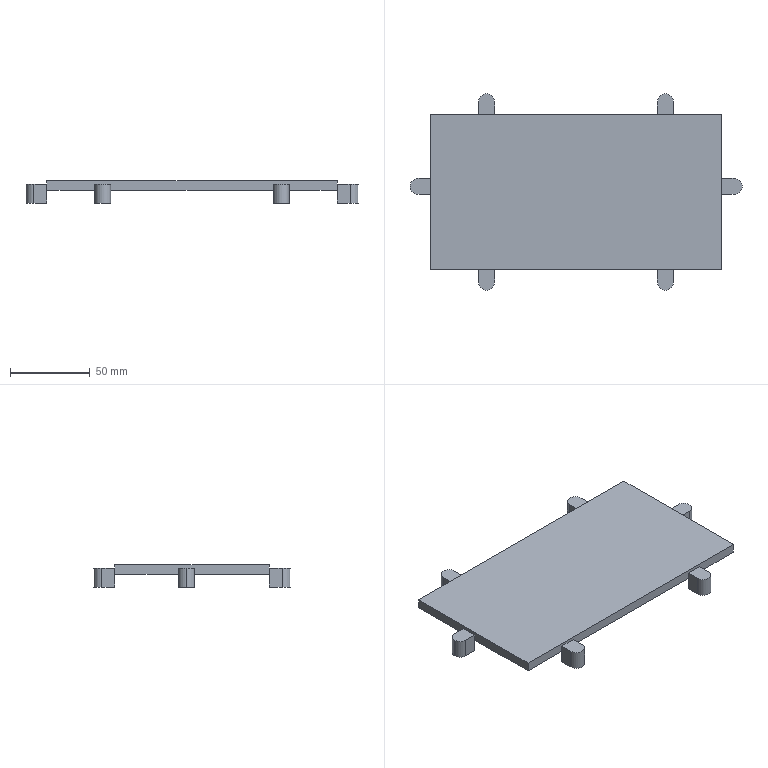Part | SolidWorks | features Extrusion 1, ICE 1 | 1 solid | 43 faces | box 208 x 123 x 14 mm | volume 114511 mm3 | plane 36 | cylinder 7 | commonest cylinder face diameters 10 x7
STEP:
#1=CARTESIAN_POINT('',(-56.993,-5.983,4.));
#2=VERTEX_POINT('',#1);
#3=CARTESIAN_POINT('',(-51.993,-10.983,4.));
#4=VERTEX_POINT('',#3);
#5=CARTESIAN_POINT('',(-51.993,-5.983,4.));
#6=DIRECTION('',(0.,0.,1.));
#7=DIRECTION('',(1.,0.,0.));
#8=AXIS2_PLACEMENT_3D('',#5,#6,#7);
#9=CIRCLE('',#8,5.);
#10=EDGE_CURVE('',#2,#4,#9,.T.);
#11=ORIENTED_EDGE('',*,*,#10,.F.);
#12=CARTESIAN_POINT('',(-56.993,-5.983,-8.));
#13=VERTEX_POINT('',#12);
#14=CARTESIAN_POINT('',(-56.993,-5.983,4.));
#15=DIRECTION('',(0.,0.,-1.));
#16=VECTOR('',#15,1000.);
#17=LINE('',#14,#16);
#18=EDGE_CURVE('',#2,#13,#17,.T.);
#19=ORIENTED_EDGE('',*,*,#18,.T.);
#20=CARTESIAN_POINT('',(-51.993,-10.983,-8.));
#21=VERTEX_POINT('',#20);
#22=CARTESIAN_POINT('',(-51.993,-5.983,-8.));
#23=DIRECTION('',(0.,0.,1.));
#24=DIRECTION('',(1.,0.,0.));
#25=AXIS2_PLACEMENT_3D('',#22,#23,#24);
#26=CIRCLE('',#25,5.);
#27=EDGE_CURVE('',#13,#21,#26,.T.);
#28=ORIENTED_EDGE('',*,*,#27,.T.);
#29=CARTESIAN_POINT('',(-51.993,-10.983,4.));
#30=DIRECTION('',(0.,0.,-1.));
#31=VECTOR('',#30,1000.);
#32=LINE('',#29,#31);
#33=EDGE_CURVE('',#4,#21,#32,.T.);
#34=ORIENTED_EDGE('',*,*,#33,.F.);
#35=EDGE_LOOP('',(#11,#19,#28,#34));
#36=FACE_OUTER_BOUND('',#35,.T.);
#37=CARTESIAN_POINT('',(-51.993,-5.983,4.));
#38=DIRECTION('',(0.,0.,-1.));
#39=DIRECTION('',(-1.,0.,0.));
#40=AXIS2_PLACEMENT_3D('',#37,#38,#39);
#41=CYLINDRICAL_SURFACE('',#40,5.);
#42=ADVANCED_FACE('',(#36),#41,.T.);
#43=CARTESIAN_POINT('',(-13.993,-57.983,4.));
#44=VERTEX_POINT('',#43);
#45=CARTESIAN_POINT('',(-13.993,-57.983,0.));
#46=VERTEX_POINT('',#45);
#47=CARTESIAN_POINT('',(-13.993,-57.983,4.));
#48=DIRECTION('',(0.,0.,-1.));
#49=VECTOR('',#48,1000.);
#50=LINE('',#47,#49);
#51=EDGE_CURVE('',#44,#46,#50,.T.);
#52=ORIENTED_EDGE('',*,*,#51,.F.);
#53=CARTESIAN_POINT('',(-3.993,-57.983,4.));
#54=VERTEX_POINT('',#53);
#55=CARTESIAN_POINT('',(-3.993,-57.983,4.));
#56=DIRECTION('',(-1.,0.,0.));
#57=VECTOR('',#56,1000.);
#58=LINE('',#55,#57);
#59=EDGE_CURVE('',#54,#44,#58,.T.);
#60=ORIENTED_EDGE('',*,*,#59,.F.);
#61=CARTESIAN_POINT('',(-3.993,-57.983,0.));
#62=VERTEX_POINT('',#61);
#63=CARTESIAN_POINT('',(-3.993,-57.983,4.));
#64=DIRECTION('',(0.,0.,-1.));
#65=VECTOR('',#64,1000.);
#66=LINE('',#63,#65);
#67=EDGE_CURVE('',#54,#62,#66,.T.);
#68=ORIENTED_EDGE('',*,*,#67,.T.);
#69=CARTESIAN_POINT('',(98.007,-57.983,0.));
#70=VERTEX_POINT('',#69);
#71=CARTESIAN_POINT('',(138.007,-57.983,0.));
#72=DIRECTION('',(1.,0.,0.));
#73=VECTOR('',#72,1000.);
#74=LINE('',#71,#73);
#75=EDGE_CURVE('',#62,#70,#74,.T.);
#76=ORIENTED_EDGE('',*,*,#75,.T.);
#77=CARTESIAN_POINT('',(98.007,-57.983,4.));
#78=VERTEX_POINT('',#77);
#79=CARTESIAN_POINT('',(98.007,-57.983,4.));
#80=DIRECTION('',(0.,0.,-1.));
#81=VECTOR('',#80,1000.);
#82=LINE('',#79,#81);
#83=EDGE_CURVE('',#78,#70,#82,.T.);
#84=ORIENTED_EDGE('',*,*,#83,.F.);
#85=CARTESIAN_POINT('',(108.007,-57.983,4.));
#86=VERTEX_POINT('',#85);
#87=CARTESIAN_POINT('',(108.007,-57.983,4.));
#88=DIRECTION('',(-1.,0.,0.));
#89=VECTOR('',#88,1000.);
#90=LINE('',#87,#89);
#91=EDGE_CURVE('',#86,#78,#90,.T.);
#92=ORIENTED_EDGE('',*,*,#91,.F.);
#93=CARTESIAN_POINT('',(108.007,-57.983,0.));
#94=VERTEX_POINT('',#93);
#95=CARTESIAN_POINT('',(108.007,-57.983,4.));
#96=DIRECTION('',(0.,0.,-1.));
#97=VECTOR('',#96,1000.);
#98=LINE('',#95,#97);
#99=EDGE_CURVE('',#86,#94,#98,.T.);
#100=ORIENTED_EDGE('',*,*,#99,.T.);
#101=CARTESIAN_POINT('',(138.007,-57.983,0.));
#102=VERTEX_POINT('',#101);
#103=CARTESIAN_POINT('',(138.007,-57.983,0.));
#104=DIRECTION('',(1.,0.,0.));
#105=VECTOR('',#104,1000.);
#106=LINE('',#103,#105);
#107=EDGE_CURVE('',#94,#102,#106,.T.);
#108=ORIENTED_EDGE('',*,*,#107,.T.);
#109=CARTESIAN_POINT('',(138.007,-57.983,6.));
#110=VERTEX_POINT('',#109);
#111=CARTESIAN_POINT('',(138.007,-57.983,6.));
#112=DIRECTION('',(0.,0.,-1.));
#113=VECTOR('',#112,1000.);
#114=LINE('',#111,#113);
#115=EDGE_CURVE('',#110,#102,#114,.T.);
#116=ORIENTED_EDGE('',*,*,#115,.F.);
#117=CARTESIAN_POINT('',(-43.993,-57.983,6.));
#118=VERTEX_POINT('',#117);
#119=CARTESIAN_POINT('',(138.007,-57.983,6.));
#120=DIRECTION('',(1.,0.,0.));
#121=VECTOR('',#120,1000.);
#122=LINE('',#119,#121);
#123=EDGE_CURVE('',#118,#110,#122,.T.);
#124=ORIENTED_EDGE('',*,*,#123,.F.);
#125=CARTESIAN_POINT('',(-43.993,-57.983,0.));
#126=VERTEX_POINT('',#125);
#127=CARTESIAN_POINT('',(-43.993,-57.983,6.));
#128=DIRECTION('',(0.,0.,-1.));
#129=VECTOR('',#128,1000.);
#130=LINE('',#127,#129);
#131=EDGE_CURVE('',#118,#126,#130,.T.);
#132=ORIENTED_EDGE('',*,*,#131,.T.);
#133=CARTESIAN_POINT('',(138.007,-57.983,0.));
#134=DIRECTION('',(1.,0.,0.));
#135=VECTOR('',#134,1000.);
#136=LINE('',#133,#135);
#137=EDGE_CURVE('',#126,#46,#136,.T.);
#138=ORIENTED_EDGE('',*,*,#137,.T.);
#139=EDGE_LOOP('',(#52,#60,#68,#76,#84,#92,#100,#108,#116,#124,#132,#138));
#140=FACE_OUTER_BOUND('',#139,.T.);
#141=CARTESIAN_POINT('',(138.007,-57.983,6.));
#142=DIRECTION('',(0.,1.,0.));
#143=DIRECTION('',(0.,0.,1.));
#144=AXIS2_PLACEMENT_3D('',#141,#142,#143);
#145=PLANE('',#144);
#146=ADVANCED_FACE('',(#140),#145,.F.);
#147=CARTESIAN_POINT('',(-43.993,-0.9829,4.));
#148=VERTEX_POINT('',#147);
#149=CARTESIAN_POINT('',(-43.993,-0.9829,0.));
#150=VERTEX_POINT('',#149);
#151=CARTESIAN_POINT('',(-43.993,-0.9829,4.));
#152=DIRECTION('',(0.,0.,-1.));
#153=VECTOR('',#152,1000.);
#154=LINE('',#151,#153);
#155=EDGE_CURVE('',#148,#150,#154,.T.);
#156=ORIENTED_EDGE('',*,*,#155,.F.);
#157=CARTESIAN_POINT('',(-43.993,-10.983,4.));
#158=VERTEX_POINT('',#157);
#159=CARTESIAN_POINT('',(-43.993,-10.983,4.));
#160=DIRECTION('',(0.,1.,0.));
#161=VECTOR('',#160,1000.);
#162=LINE('',#159,#161);
#163=EDGE_CURVE('',#158,#148,#162,.T.);
#164=ORIENTED_EDGE('',*,*,#163,.F.);
#165=CARTESIAN_POINT('',(-43.993,-10.983,0.));
#166=VERTEX_POINT('',#165);
#167=CARTESIAN_POINT('',(-43.993,-10.983,4.));
#168=DIRECTION('',(0.,0.,-1.));
#169=VECTOR('',#168,1000.);
#170=LINE('',#167,#169);
#171=EDGE_CURVE('',#158,#166,#170,.T.);
#172=ORIENTED_EDGE('',*,*,#171,.T.);
#173=CARTESIAN_POINT('',(-43.993,-57.983,0.));
#174=DIRECTION('',(0.,-1.,0.));
#175=VECTOR('',#174,1000.);
#176=LINE('',#173,#175);
#177=EDGE_CURVE('',#166,#126,#176,.T.);
#178=ORIENTED_EDGE('',*,*,#177,.T.);
#179=ORIENTED_EDGE('',*,*,#131,.F.);
#180=CARTESIAN_POINT('',(-43.993,39.017,6.));
#181=VERTEX_POINT('',#180);
#182=CARTESIAN_POINT('',(-43.993,-57.983,6.));
#183=DIRECTION('',(0.,-1.,0.));
#184=VECTOR('',#183,1000.);
#185=LINE('',#182,#184);
#186=EDGE_CURVE('',#181,#118,#185,.T.);
#187=ORIENTED_EDGE('',*,*,#186,.F.);
#188=CARTESIAN_POINT('',(-43.993,39.017,0.));
#189=VERTEX_POINT('',#188);
#190=CARTESIAN_POINT('',(-43.993,39.017,6.));
#191=DIRECTION('',(0.,0.,-1.));
#192=VECTOR('',#191,1000.);
#193=LINE('',#190,#192);
#194=EDGE_CURVE('',#181,#189,#193,.T.);
#195=ORIENTED_EDGE('',*,*,#194,.T.);
#196=CARTESIAN_POINT('',(-43.993,-57.983,0.));
#197=DIRECTION('',(0.,-1.,0.));
#198=VECTOR('',#197,1000.);
#199=LINE('',#196,#198);
#200=EDGE_CURVE('',#189,#150,#199,.T.);
#201=ORIENTED_EDGE('',*,*,#200,.T.);
#202=EDGE_LOOP('',(#156,#164,#172,#178,#179,#187,#195,#201));
#203=FACE_OUTER_BOUND('',#202,.T.);
#204=CARTESIAN_POINT('',(-43.993,-57.983,6.));
#205=DIRECTION('',(1.,0.,0.));
#206=DIRECTION('',(0.,0.,-1.));
#207=AXIS2_PLACEMENT_3D('',#204,#205,#206);
#208=PLANE('',#207);
#209=ADVANCED_FACE('',(#203),#208,.F.);
#210=CARTESIAN_POINT('',(108.007,39.017,4.));
#211=VERTEX_POINT('',#210);
#212=CARTESIAN_POINT('',(108.007,39.017,0.));
#213=VERTEX_POINT('',#212);
#214=CARTESIAN_POINT('',(108.007,39.017,4.));
#215=DIRECTION('',(0.,0.,-1.));
#216=VECTOR('',#215,1000.);
#217=LINE('',#214,#216);
#218=EDGE_CURVE('',#211,#213,#217,.T.);
#219=ORIENTED_EDGE('',*,*,#218,.F.);
#220=CARTESIAN_POINT('',(98.007,39.017,4.));
#221=VERTEX_POINT('',#220);
#222=CARTESIAN_POINT('',(98.007,39.017,4.));
#223=DIRECTION('',(1.,0.,0.));
#224=VECTOR('',#223,1000.);
#225=LINE('',#222,#224);
#226=EDGE_CURVE('',#221,#211,#225,.T.);
#227=ORIENTED_EDGE('',*,*,#226,.F.);
#228=CARTESIAN_POINT('',(98.007,39.017,0.));
#229=VERTEX_POINT('',#228);
#230=CARTESIAN_POINT('',(98.007,39.017,4.));
#231=DIRECTION('',(0.,0.,-1.));
#232=VECTOR('',#231,1000.);
#233=LINE('',#230,#232);
#234=EDGE_CURVE('',#221,#229,#233,.T.);
#235=ORIENTED_EDGE('',*,*,#234,.T.);
#236=CARTESIAN_POINT('',(-3.993,39.017,0.));
#237=VERTEX_POINT('',#236);
#238=CARTESIAN_POINT('',(138.007,39.017,0.));
#239=DIRECTION('',(-1.,0.,0.));
#240=VECTOR('',#239,1000.);
#241=LINE('',#238,#240);
#242=EDGE_CURVE('',#229,#237,#241,.T.);
#243=ORIENTED_EDGE('',*,*,#242,.T.);
#244=CARTESIAN_POINT('',(-3.993,39.017,4.));
#245=VERTEX_POINT('',#244);
#246=CARTESIAN_POINT('',(-3.993,39.017,4.));
#247=DIRECTION('',(0.,0.,-1.));
#248=VECTOR('',#247,1000.);
#249=LINE('',#246,#248);
#250=EDGE_CURVE('',#245,#237,#249,.T.);
#251=ORIENTED_EDGE('',*,*,#250,.F.);
#252=CARTESIAN_POINT('',(-13.993,39.017,4.));
#253=VERTEX_POINT('',#252);
#254=CARTESIAN_POINT('',(-13.993,39.017,4.));
#255=DIRECTION('',(1.,0.,0.));
#256=VECTOR('',#255,1000.);
#257=LINE('',#254,#256);
#258=EDGE_CURVE('',#253,#245,#257,.T.);
#259=ORIENTED_EDGE('',*,*,#258,.F.);
#260=CARTESIAN_POINT('',(-13.993,39.017,0.));
#261=VERTEX_POINT('',#260);
#262=CARTESIAN_POINT('',(-13.993,39.017,4.));
#263=DIRECTION('',(0.,0.,-1.));
#264=VECTOR('',#263,1000.);
#265=LINE('',#262,#264);
#266=EDGE_CURVE('',#253,#261,#265,.T.);
#267=ORIENTED_EDGE('',*,*,#266,.T.);
#268=CARTESIAN_POINT('',(138.007,39.017,0.));
#269=DIRECTION('',(-1.,0.,0.));
#270=VECTOR('',#269,1000.);
#271=LINE('',#268,#270);
#272=EDGE_CURVE('',#261,#189,#271,.T.);
#273=ORIENTED_EDGE('',*,*,#272,.T.);
#274=ORIENTED_EDGE('',*,*,#194,.F.);
#275=CARTESIAN_POINT('',(138.007,39.017,6.));
#276=VERTEX_POINT('',#275);
#277=CARTESIAN_POINT('',(138.007,39.017,6.));
#278=DIRECTION('',(-1.,0.,0.));
#279=VECTOR('',#278,1000.);
#280=LINE('',#277,#279);
#281=EDGE_CURVE('',#276,#181,#280,.T.);
#282=ORIENTED_EDGE('',*,*,#281,.F.);
#283=CARTESIAN_POINT('',(138.007,39.017,0.));
#284=VERTEX_POINT('',#283);
#285=CARTESIAN_POINT('',(138.007,39.017,6.));
#286=DIRECTION('',(0.,0.,-1.));
#287=VECTOR('',#286,1000.);
#288=LINE('',#285,#287);
#289=EDGE_CURVE('',#276,#284,#288,.T.);
#290=ORIENTED_EDGE('',*,*,#289,.T.);
#291=CARTESIAN_POINT('',(138.007,39.017,0.));
#292=DIRECTION('',(-1.,0.,0.));
#293=VECTOR('',#292,1000.);
#294=LINE('',#291,#293);
#295=EDGE_CURVE('',#284,#213,#294,.T.);
#296=ORIENTED_EDGE('',*,*,#295,.T.);
#297=EDGE_LOOP('',(#219,#227,#235,#243,#251,#259,#267,#273,#274,#282,#290,#296));
#298=FACE_OUTER_BOUND('',#297,.T.);
#299=CARTESIAN_POINT('',(138.007,39.017,6.));
#300=DIRECTION('',(0.,-1.,0.));
#301=DIRECTION('',(0.,0.,-1.));
#302=AXIS2_PLACEMENT_3D('',#299,#300,#301);
#303=PLANE('',#302);
#304=ADVANCED_FACE('',(#298),#303,.F.);
#305=CARTESIAN_POINT('',(138.007,-10.983,4.));
#306=VERTEX_POINT('',#305);
#307=CARTESIAN_POINT('',(138.007,-10.983,0.));
#308=VERTEX_POINT('',#307);
#309=CARTESIAN_POINT('',(138.007,-10.983,4.));
#310=DIRECTION('',(0.,0.,-1.));
#311=VECTOR('',#310,1000.);
#312=LINE('',#309,#311);
#313=EDGE_CURVE('',#306,#308,#312,.T.);
#314=ORIENTED_EDGE('',*,*,#313,.F.);
#315=CARTESIAN_POINT('',(138.007,-0.9829,4.));
#316=VERTEX_POINT('',#315);
#317=CARTESIAN_POINT('',(138.007,-0.9829,4.));
#318=DIRECTION('',(0.,-1.,0.));
#319=VECTOR('',#318,1000.);
#320=LINE('',#317,#319);
#321=EDGE_CURVE('',#316,#306,#320,.T.);
#322=ORIENTED_EDGE('',*,*,#321,.F.);
#323=CARTESIAN_POINT('',(138.007,-0.9829,0.));
#324=VERTEX_POINT('',#323);
#325=CARTESIAN_POINT('',(138.007,-0.9829,4.));
#326=DIRECTION('',(0.,0.,-1.));
#327=VECTOR('',#326,1000.);
#328=LINE('',#325,#327);
#329=EDGE_CURVE('',#316,#324,#328,.T.);
#330=ORIENTED_EDGE('',*,*,#329,.T.);
#331=CARTESIAN_POINT('',(138.007,-57.983,0.));
#332=DIRECTION('',(0.,1.,0.));
#333=VECTOR('',#332,1000.);
#334=LINE('',#331,#333);
#335=EDGE_CURVE('',#324,#284,#334,.T.);
#336=ORIENTED_EDGE('',*,*,#335,.T.);
#337=ORIENTED_EDGE('',*,*,#289,.F.);
#338=CARTESIAN_POINT('',(138.007,-57.983,6.));
#339=DIRECTION('',(0.,1.,0.));
#340=VECTOR('',#339,1000.);
#341=LINE('',#338,#340);
#342=EDGE_CURVE('',#110,#276,#341,.T.);
#343=ORIENTED_EDGE('',*,*,#342,.F.);
#344=ORIENTED_EDGE('',*,*,#115,.T.);
#345=CARTESIAN_POINT('',(138.007,-57.983,0.));
#346=DIRECTION('',(0.,1.,0.));
#347=VECTOR('',#346,1000.);
#348=LINE('',#345,#347);
#349=EDGE_CURVE('',#102,#308,#348,.T.);
#350=ORIENTED_EDGE('',*,*,#349,.T.);
#351=EDGE_LOOP('',(#314,#322,#330,#336,#337,#343,#344,#350));
#352=FACE_OUTER_BOUND('',#351,.T.);
#353=CARTESIAN_POINT('',(138.007,-57.983,6.));
#354=DIRECTION('',(-1.,0.,0.));
#355=DIRECTION('',(0.,0.,1.));
#356=AXIS2_PLACEMENT_3D('',#353,#354,#355);
#357=PLANE('',#356);
#358=ADVANCED_FACE('',(#352),#357,.F.);
#359=ORIENTED_EDGE('',*,*,#342,.T.);
#360=ORIENTED_EDGE('',*,*,#281,.T.);
#361=ORIENTED_EDGE('',*,*,#186,.T.);
#362=ORIENTED_EDGE('',*,*,#123,.T.);
#363=EDGE_LOOP('',(#359,#360,#361,#362));
#364=FACE_OUTER_BOUND('',#363,.T.);
#365=CARTESIAN_POINT('',(0.,0.,6.));
#366=DIRECTION('',(0.,0.,1.));
#367=DIRECTION('',(1.,0.,0.));
#368=AXIS2_PLACEMENT_3D('',#365,#366,#367);
#369=PLANE('',#368);
#370=ADVANCED_FACE('',(#364),#369,.T.);
#371=ORIENTED_EDGE('',*,*,#349,.F.);
#372=ORIENTED_EDGE('',*,*,#107,.F.);
#373=CARTESIAN_POINT('',(138.007,-57.983,0.));
#374=DIRECTION('',(1.,0.,0.));
#375=VECTOR('',#374,1000.);
#376=LINE('',#373,#375);
#377=EDGE_CURVE('',#70,#94,#376,.T.);
#378=ORIENTED_EDGE('',*,*,#377,.F.);
#379=ORIENTED_EDGE('',*,*,#75,.F.);
#380=CARTESIAN_POINT('',(138.007,-57.983,0.));
#381=DIRECTION('',(1.,0.,0.));
#382=VECTOR('',#381,1000.);
#383=LINE('',#380,#382);
#384=EDGE_CURVE('',#46,#62,#383,.T.);
#385=ORIENTED_EDGE('',*,*,#384,.F.);
#386=ORIENTED_EDGE('',*,*,#137,.F.);
#387=ORIENTED_EDGE('',*,*,#177,.F.);
#388=CARTESIAN_POINT('',(-43.993,-57.983,0.));
#389=DIRECTION('',(0.,-1.,0.));
#390=VECTOR('',#389,1000.);
#391=LINE('',#388,#390);
#392=EDGE_CURVE('',#150,#166,#391,.T.);
#393=ORIENTED_EDGE('',*,*,#392,.F.);
#394=ORIENTED_EDGE('',*,*,#200,.F.);
#395=ORIENTED_EDGE('',*,*,#272,.F.);
#396=CARTESIAN_POINT('',(138.007,39.017,0.));
#397=DIRECTION('',(-1.,0.,0.));
#398=VECTOR('',#397,1000.);
#399=LINE('',#396,#398);
#400=EDGE_CURVE('',#237,#261,#399,.T.);
#401=ORIENTED_EDGE('',*,*,#400,.F.);
#402=ORIENTED_EDGE('',*,*,#242,.F.);
#403=CARTESIAN_POINT('',(138.007,39.017,0.));
#404=DIRECTION('',(-1.,0.,0.));
#405=VECTOR('',#404,1000.);
#406=LINE('',#403,#405);
#407=EDGE_CURVE('',#213,#229,#406,.T.);
#408=ORIENTED_EDGE('',*,*,#407,.F.);
#409=ORIENTED_EDGE('',*,*,#295,.F.);
#410=ORIENTED_EDGE('',*,*,#335,.F.);
#411=CARTESIAN_POINT('',(138.007,-57.983,0.));
#412=DIRECTION('',(0.,1.,0.));
#413=VECTOR('',#412,1000.);
#414=LINE('',#411,#413);
#415=EDGE_CURVE('',#308,#324,#414,.T.);
#416=ORIENTED_EDGE('',*,*,#415,.F.);
#417=EDGE_LOOP('',(#371,#372,#378,#379,#385,#386,#387,#393,#394,#395,#401,#402,#408,#409,#410,#416));
#418=FACE_OUTER_BOUND('',#417,.T.);
#419=CARTESIAN_POINT('',(0.,0.,0.));
#420=DIRECTION('',(0.,0.,1.));
#421=DIRECTION('',(1.,0.,0.));
#422=AXIS2_PLACEMENT_3D('',#419,#420,#421);
#423=PLANE('',#422);
#424=ADVANCED_FACE('',(#418),#423,.F.);
#425=CARTESIAN_POINT('',(98.007,-57.983,-8.));
#426=VERTEX_POINT('',#425);
#427=CARTESIAN_POINT('',(98.007,-57.983,4.));
#428=DIRECTION('',(0.,0.,-1.));
#429=VECTOR('',#428,1000.);
#430=LINE('',#427,#429);
#431=EDGE_CURVE('',#70,#426,#430,.T.);
#432=ORIENTED_EDGE('',*,*,#431,.F.);
#433=ORIENTED_EDGE('',*,*,#377,.T.);
#434=CARTESIAN_POINT('',(108.007,-57.983,-8.));
#435=VERTEX_POINT('',#434);
#436=CARTESIAN_POINT('',(108.007,-57.983,4.));
#437=DIRECTION('',(0.,0.,-1.));
#438=VECTOR('',#437,1000.);
#439=LINE('',#436,#438);
#440=EDGE_CURVE('',#94,#435,#439,.T.);
#441=ORIENTED_EDGE('',*,*,#440,.T.);
#442=CARTESIAN_POINT('',(108.007,-57.983,-8.));
#443=DIRECTION('',(-1.,0.,0.));
#444=VECTOR('',#443,1000.);
#445=LINE('',#442,#444);
#446=EDGE_CURVE('',#435,#426,#445,.T.);
#447=ORIENTED_EDGE('',*,*,#446,.T.);
#448=EDGE_LOOP('',(#432,#433,#441,#447));
#449=FACE_OUTER_BOUND('',#448,.T.);
#450=CARTESIAN_POINT('',(108.007,-57.983,4.));
#451=DIRECTION('',(0.,-1.,0.));
#452=DIRECTION('',(0.,0.,-1.));
#453=AXIS2_PLACEMENT_3D('',#450,#451,#452);
#454=PLANE('',#453);
#455=ADVANCED_FACE('',(#449),#454,.F.);
#456=CARTESIAN_POINT('',(98.007,-65.983,-8.));
#457=VERTEX_POINT('',#456);
#458=CARTESIAN_POINT('',(108.007,-65.983,-8.));
#459=VERTEX_POINT('',#458);
#460=CARTESIAN_POINT('',(103.007,-65.983,-8.));
#461=DIRECTION('',(0.,0.,1.));
#462=DIRECTION('',(1.,0.,0.));
#463=AXIS2_PLACEMENT_3D('',#460,#461,#462);
#464=CIRCLE('',#463,5.);
#465=EDGE_CURVE('',#457,#459,#464,.T.);
#466=ORIENTED_EDGE('',*,*,#465,.T.);
#467=CARTESIAN_POINT('',(108.007,-65.983,4.));
#468=VERTEX_POINT('',#467);
#469=CARTESIAN_POINT('',(108.007,-65.983,4.));
#470=DIRECTION('',(0.,0.,-1.));
#471=VECTOR('',#470,1000.);
#472=LINE('',#469,#471);
#473=EDGE_CURVE('',#468,#459,#472,.T.);
#474=ORIENTED_EDGE('',*,*,#473,.F.);
#475=CARTESIAN_POINT('',(98.007,-65.983,4.));
#476=VERTEX_POINT('',#475);
#477=CARTESIAN_POINT('',(103.007,-65.983,4.));
#478=DIRECTION('',(0.,0.,1.));
#479=DIRECTION('',(1.,0.,0.));
#480=AXIS2_PLACEMENT_3D('',#477,#478,#479);
#481=CIRCLE('',#480,5.);
#482=EDGE_CURVE('',#476,#468,#481,.T.);
#483=ORIENTED_EDGE('',*,*,#482,.F.);
#484=CARTESIAN_POINT('',(98.007,-65.983,4.));
#485=DIRECTION('',(0.,0.,-1.));
#486=VECTOR('',#485,1000.);
#487=LINE('',#484,#486);
#488=EDGE_CURVE('',#476,#457,#487,.T.);
#489=ORIENTED_EDGE('',*,*,#488,.T.);
#490=EDGE_LOOP('',(#466,#474,#483,#489));
#491=FACE_OUTER_BOUND('',#490,.T.);
#492=CARTESIAN_POINT('',(103.007,-65.983,4.));
#493=DIRECTION('',(0.,0.,-1.));
#494=DIRECTION('',(-1.,0.,0.));
#495=AXIS2_PLACEMENT_3D('',#492,#493,#494);
#496=CYLINDRICAL_SURFACE('',#495,5.);
#497=ADVANCED_FACE('',(#491),#496,.T.);
#498=CARTESIAN_POINT('',(108.007,-65.983,-8.));
#499=DIRECTION('',(0.,1.,0.));
#500=VECTOR('',#499,1000.);
#501=LINE('',#498,#500);
#502=EDGE_CURVE('',#459,#435,#501,.T.);
#503=ORIENTED_EDGE('',*,*,#502,.T.);
#504=ORIENTED_EDGE('',*,*,#440,.F.);
#505=ORIENTED_EDGE('',*,*,#99,.F.);
#506=CARTESIAN_POINT('',(108.007,-65.983,4.));
#507=DIRECTION('',(0.,1.,0.));
#508=VECTOR('',#507,1000.);
#509=LINE('',#506,#508);
#510=EDGE_CURVE('',#468,#86,#509,.T.);
#511=ORIENTED_EDGE('',*,*,#510,.F.);
#512=ORIENTED_EDGE('',*,*,#473,.T.);
#513=EDGE_LOOP('',(#503,#504,#505,#511,#512));
#514=FACE_OUTER_BOUND('',#513,.T.);
#515=CARTESIAN_POINT('',(108.007,-65.983,4.));
#516=DIRECTION('',(-1.,0.,0.));
#517=DIRECTION('',(0.,-1.,0.));
#518=AXIS2_PLACEMENT_3D('',#515,#516,#517);
#519=PLANE('',#518);
#520=ADVANCED_FACE('',(#514),#519,.F.);
#521=CARTESIAN_POINT('',(98.007,-57.983,-8.));
#522=DIRECTION('',(0.,-1.,0.));
#523=VECTOR('',#522,1000.);
#524=LINE('',#521,#523);
#525=EDGE_CURVE('',#426,#457,#524,.T.);
#526=ORIENTED_EDGE('',*,*,#525,.T.);
#527=ORIENTED_EDGE('',*,*,#488,.F.);
#528=CARTESIAN_POINT('',(98.007,-57.983,4.));
#529=DIRECTION('',(0.,-1.,0.));
#530=VECTOR('',#529,1000.);
#531=LINE('',#528,#530);
#532=EDGE_CURVE('',#78,#476,#531,.T.);
#533=ORIENTED_EDGE('',*,*,#532,.F.);
#534=ORIENTED_EDGE('',*,*,#83,.T.);
#535=ORIENTED_EDGE('',*,*,#431,.T.);
#536=EDGE_LOOP('',(#526,#527,#533,#534,#535));
#537=FACE_OUTER_BOUND('',#536,.T.);
#538=CARTESIAN_POINT('',(98.007,-57.983,4.));
#539=DIRECTION('',(1.,0.,0.));
#540=DIRECTION('',(0.,1.,0.));
#541=AXIS2_PLACEMENT_3D('',#538,#539,#540);
#542=PLANE('',#541);
#543=ADVANCED_FACE('',(#537),#542,.F.);
#544=ORIENTED_EDGE('',*,*,#482,.T.);
#545=ORIENTED_EDGE('',*,*,#510,.T.);
#546=ORIENTED_EDGE('',*,*,#91,.T.);
#547=ORIENTED_EDGE('',*,*,#532,.T.);
#548=EDGE_LOOP('',(#544,#545,#546,#547));
#549=FACE_OUTER_BOUND('',#548,.T.);
#550=CARTESIAN_POINT('',(103.007,-65.983,4.));
#551=DIRECTION('',(0.,0.,1.));
#552=DIRECTION('',(1.,0.,0.));
#553=AXIS2_PLACEMENT_3D('',#550,#551,#552);
#554=PLANE('',#553);
#555=ADVANCED_FACE('',(#549),#554,.T.);
#556=ORIENTED_EDGE('',*,*,#465,.F.);
#557=ORIENTED_EDGE('',*,*,#525,.F.);
#558=ORIENTED_EDGE('',*,*,#446,.F.);
#559=ORIENTED_EDGE('',*,*,#502,.F.);
#560=EDGE_LOOP('',(#556,#557,#558,#559));
#561=FACE_OUTER_BOUND('',#560,.T.);
#562=CARTESIAN_POINT('',(103.007,-65.983,-8.));
#563=DIRECTION('',(0.,0.,1.));
#564=DIRECTION('',(1.,0.,0.));
#565=AXIS2_PLACEMENT_3D('',#562,#563,#564);
#566=PLANE('',#565);
#567=ADVANCED_FACE('',(#561),#566,.F.);
#568=CARTESIAN_POINT('',(138.007,-10.983,-8.));
#569=VERTEX_POINT('',#568);
#570=CARTESIAN_POINT('',(138.007,-10.983,4.));
#571=DIRECTION('',(0.,0.,-1.));
#572=VECTOR('',#571,1000.);
#573=LINE('',#570,#572);
#574=EDGE_CURVE('',#308,#569,#573,.T.);
#575=ORIENTED_EDGE('',*,*,#574,.F.);
#576=ORIENTED_EDGE('',*,*,#415,.T.);
#577=CARTESIAN_POINT('',(138.007,-0.9829,-8.));
#578=VERTEX_POINT('',#577);
#579=CARTESIAN_POINT('',(138.007,-0.9829,4.));
#580=DIRECTION('',(0.,0.,-1.));
#581=VECTOR('',#580,1000.);
#582=LINE('',#579,#581);
#583=EDGE_CURVE('',#324,#578,#582,.T.);
#584=ORIENTED_EDGE('',*,*,#583,.T.);
#585=CARTESIAN_POINT('',(138.007,-0.9829,-8.));
#586=DIRECTION('',(0.,-1.,0.));
#587=VECTOR('',#586,1000.);
#588=LINE('',#585,#587);
#589=EDGE_CURVE('',#578,#569,#588,.T.);
#590=ORIENTED_EDGE('',*,*,#589,.T.);
#591=EDGE_LOOP('',(#575,#576,#584,#590));
#592=FACE_OUTER_BOUND('',#591,.T.);
#593=CARTESIAN_POINT('',(138.007,-0.9829,4.));
#594=DIRECTION('',(1.,0.,0.));
#595=DIRECTION('',(0.,0.,-1.));
#596=AXIS2_PLACEMENT_3D('',#593,#594,#595);
#597=PLANE('',#596);
#598=ADVANCED_FACE('',(#592),#597,.F.);
#599=CARTESIAN_POINT('',(146.007,-0.9829,-8.));
#600=VERTEX_POINT('',#599);
#601=CARTESIAN_POINT('',(146.007,-0.9829,-8.));
#602=DIRECTION('',(-1.,0.,0.));
#603=VECTOR('',#602,1000.);
#604=LINE('',#601,#603);
#605=EDGE_CURVE('',#600,#578,#604,.T.);
#606=ORIENTED_EDGE('',*,*,#605,.T.);
#607=ORIENTED_EDGE('',*,*,#583,.F.);
#608=ORIENTED_EDGE('',*,*,#329,.F.);
#609=CARTESIAN_POINT('',(146.007,-0.9829,4.));
#610=VERTEX_POINT('',#609);
#611=CARTESIAN_POINT('',(146.007,-0.9829,4.));
#612=DIRECTION('',(-1.,0.,0.));
#613=VECTOR('',#612,1000.);
#614=LINE('',#611,#613);
#615=EDGE_CURVE('',#610,#316,#614,.T.);
#616=ORIENTED_EDGE('',*,*,#615,.F.);
#617=CARTESIAN_POINT('',(146.007,-0.9829,4.));
#618=DIRECTION('',(0.,0.,-1.));
#619=VECTOR('',#618,1000.);
#620=LINE('',#617,#619);
#621=EDGE_CURVE('',#610,#600,#620,.T.);
#622=ORIENTED_EDGE('',*,*,#621,.T.);
#623=EDGE_LOOP('',(#606,#607,#608,#616,#622));
#624=FACE_OUTER_BOUND('',#623,.T.);
#625=CARTESIAN_POINT('',(146.007,-0.9829,4.));
#626=DIRECTION('',(0.,-1.,0.));
#627=DIRECTION('',(0.,0.,-1.));
#628=AXIS2_PLACEMENT_3D('',#625,#626,#627);
#629=PLANE('',#628);
#630=ADVANCED_FACE('',(#624),#629,.F.);
#631=CARTESIAN_POINT('',(146.007,-10.983,-8.));
#632=VERTEX_POINT('',#631);
#633=CARTESIAN_POINT('',(138.007,-10.983,-8.));
#634=DIRECTION('',(1.,0.,0.));
#635=VECTOR('',#634,1000.);
#636=LINE('',#633,#635);
#637=EDGE_CURVE('',#569,#632,#636,.T.);
#638=ORIENTED_EDGE('',*,*,#637,.T.);
#639=CARTESIAN_POINT('',(146.007,-10.983,4.));
#640=VERTEX_POINT('',#639);
#641=CARTESIAN_POINT('',(146.007,-10.983,4.));
#642=DIRECTION('',(0.,0.,-1.));
#643=VECTOR('',#642,1000.);
#644=LINE('',#641,#643);
#645=EDGE_CURVE('',#640,#632,#644,.T.);
#646=ORIENTED_EDGE('',*,*,#645,.F.);
#647=CARTESIAN_POINT('',(138.007,-10.983,4.));
#648=DIRECTION('',(1.,0.,0.));
#649=VECTOR('',#648,1000.);
#650=LINE('',#647,#649);
#651=EDGE_CURVE('',#306,#640,#650,.T.);
#652=ORIENTED_EDGE('',*,*,#651,.F.);
#653=ORIENTED_EDGE('',*,*,#313,.T.);
#654=ORIENTED_EDGE('',*,*,#574,.T.);
#655=EDGE_LOOP('',(#638,#646,#652,#653,#654));
#656=FACE_OUTER_BOUND('',#655,.T.);
#657=CARTESIAN_POINT('',(138.007,-10.983,4.));
#658=DIRECTION('',(0.,1.,0.));
#659=DIRECTION('',(-1.,0.,0.));
#660=AXIS2_PLACEMENT_3D('',#657,#658,#659);
#661=PLANE('',#660);
#662=ADVANCED_FACE('',(#656),#661,.F.);
#663=CARTESIAN_POINT('',(146.007,-5.983,-8.));
#664=DIRECTION('',(0.,0.,1.));
#665=DIRECTION('',(1.,0.,0.));
#666=AXIS2_PLACEMENT_3D('',#663,#664,#665);
#667=CIRCLE('',#666,5.);
#668=EDGE_CURVE('',#632,#600,#667,.T.);
#669=ORIENTED_EDGE('',*,*,#668,.T.);
#670=ORIENTED_EDGE('',*,*,#621,.F.);
#671=CARTESIAN_POINT('',(146.007,-5.983,4.));
#672=DIRECTION('',(0.,0.,1.));
#673=DIRECTION('',(1.,0.,0.));
#674=AXIS2_PLACEMENT_3D('',#671,#672,#673);
#675=CIRCLE('',#674,5.);
#676=EDGE_CURVE('',#640,#610,#675,.T.);
#677=ORIENTED_EDGE('',*,*,#676,.F.);
#678=ORIENTED_EDGE('',*,*,#645,.T.);
#679=EDGE_LOOP('',(#669,#670,#677,#678));
#680=FACE_OUTER_BOUND('',#679,.T.);
#681=CARTESIAN_POINT('',(146.007,-5.983,4.));
#682=DIRECTION('',(0.,0.,-1.));
#683=DIRECTION('',(-1.,0.,0.));
#684=AXIS2_PLACEMENT_3D('',#681,#682,#683);
#685=CYLINDRICAL_SURFACE('',#684,5.);
#686=ADVANCED_FACE('',(#680),#685,.T.);
#687=ORIENTED_EDGE('',*,*,#615,.T.);
#688=ORIENTED_EDGE('',*,*,#321,.T.);
#689=ORIENTED_EDGE('',*,*,#651,.T.);
#690=ORIENTED_EDGE('',*,*,#676,.T.);
#691=EDGE_LOOP('',(#687,#688,#689,#690));
#692=FACE_OUTER_BOUND('',#691,.T.);
#693=CARTESIAN_POINT('',(146.007,-5.983,4.));
#694=DIRECTION('',(0.,0.,1.));
#695=DIRECTION('',(1.,0.,0.));
#696=AXIS2_PLACEMENT_3D('',#693,#694,#695);
#697=PLANE('',#696);
#698=ADVANCED_FACE('',(#692),#697,.T.);
#699=ORIENTED_EDGE('',*,*,#605,.F.);
#700=ORIENTED_EDGE('',*,*,#668,.F.);
#701=ORIENTED_EDGE('',*,*,#637,.F.);
#702=ORIENTED_EDGE('',*,*,#589,.F.);
#703=EDGE_LOOP('',(#699,#700,#701,#702));
#704=FACE_OUTER_BOUND('',#703,.T.);
#705=CARTESIAN_POINT('',(146.007,-5.983,-8.));
#706=DIRECTION('',(0.,0.,1.));
#707=DIRECTION('',(1.,0.,0.));
#708=AXIS2_PLACEMENT_3D('',#705,#706,#707);
#709=PLANE('',#708);
#710=ADVANCED_FACE('',(#704),#709,.F.);
#711=CARTESIAN_POINT('',(-3.993,39.017,-8.));
#712=VERTEX_POINT('',#711);
#713=CARTESIAN_POINT('',(-3.993,39.017,4.));
#714=DIRECTION('',(0.,0.,-1.));
#715=VECTOR('',#714,1000.);
#716=LINE('',#713,#715);
#717=EDGE_CURVE('',#237,#712,#716,.T.);
#718=ORIENTED_EDGE('',*,*,#717,.F.);
#719=ORIENTED_EDGE('',*,*,#400,.T.);
#720=CARTESIAN_POINT('',(-13.993,39.017,-8.));
#721=VERTEX_POINT('',#720);
#722=CARTESIAN_POINT('',(-13.993,39.017,4.));
#723=DIRECTION('',(0.,0.,-1.));
#724=VECTOR('',#723,1000.);
#725=LINE('',#722,#724);
#726=EDGE_CURVE('',#261,#721,#725,.T.);
#727=ORIENTED_EDGE('',*,*,#726,.T.);
#728=CARTESIAN_POINT('',(-13.993,39.017,-8.));
#729=DIRECTION('',(1.,0.,0.));
#730=VECTOR('',#729,1000.);
#731=LINE('',#728,#730);
#732=EDGE_CURVE('',#721,#712,#731,.T.);
#733=ORIENTED_EDGE('',*,*,#732,.T.);
#734=EDGE_LOOP('',(#718,#719,#727,#733));
#735=FACE_OUTER_BOUND('',#734,.T.);
#736=CARTESIAN_POINT('',(-13.993,39.017,4.));
#737=DIRECTION('',(0.,1.,0.));
#738=DIRECTION('',(0.,0.,1.));
#739=AXIS2_PLACEMENT_3D('',#736,#737,#738);
#740=PLANE('',#739);
#741=ADVANCED_FACE('',(#735),#740,.F.);
#742=CARTESIAN_POINT('',(-3.993,47.017,-8.));
#743=VERTEX_POINT('',#742);
#744=CARTESIAN_POINT('',(-13.993,47.017,-8.));
#745=VERTEX_POINT('',#744);
#746=CARTESIAN_POINT('',(-8.993,47.017,-8.));
#747=DIRECTION('',(0.,0.,1.));
#748=DIRECTION('',(1.,0.,0.));
#749=AXIS2_PLACEMENT_3D('',#746,#747,#748);
#750=CIRCLE('',#749,5.);
#751=EDGE_CURVE('',#743,#745,#750,.T.);
#752=ORIENTED_EDGE('',*,*,#751,.T.);
#753=CARTESIAN_POINT('',(-13.993,47.017,4.));
#754=VERTEX_POINT('',#753);
#755=CARTESIAN_POINT('',(-13.993,47.017,4.));
#756=DIRECTION('',(0.,0.,-1.));
#757=VECTOR('',#756,1000.);
#758=LINE('',#755,#757);
#759=EDGE_CURVE('',#754,#745,#758,.T.);
#760=ORIENTED_EDGE('',*,*,#759,.F.);
#761=CARTESIAN_POINT('',(-3.993,47.017,4.));
#762=VERTEX_POINT('',#761);
#763=CARTESIAN_POINT('',(-8.993,47.017,4.));
#764=DIRECTION('',(0.,0.,1.));
#765=DIRECTION('',(1.,0.,0.));
#766=AXIS2_PLACEMENT_3D('',#763,#764,#765);
#767=CIRCLE('',#766,5.);
#768=EDGE_CURVE('',#762,#754,#767,.T.);
#769=ORIENTED_EDGE('',*,*,#768,.F.);
#770=CARTESIAN_POINT('',(-3.993,47.017,4.));
#771=DIRECTION('',(0.,0.,-1.));
#772=VECTOR('',#771,1000.);
#773=LINE('',#770,#772);
#774=EDGE_CURVE('',#762,#743,#773,.T.);
#775=ORIENTED_EDGE('',*,*,#774,.T.);
#776=EDGE_LOOP('',(#752,#760,#769,#775));
#777=FACE_OUTER_BOUND('',#776,.T.);
#778=CARTESIAN_POINT('',(-8.993,47.017,4.));
#779=DIRECTION('',(0.,0.,-1.));
#780=DIRECTION('',(-1.,0.,0.));
#781=AXIS2_PLACEMENT_3D('',#778,#779,#780);
#782=CYLINDRICAL_SURFACE('',#781,5.);
#783=ADVANCED_FACE('',(#777),#782,.T.);
#784=CARTESIAN_POINT('',(-13.993,47.017,-8.));
#785=DIRECTION('',(0.,-1.,0.));
#786=VECTOR('',#785,1000.);
#787=LINE('',#784,#786);
#788=EDGE_CURVE('',#745,#721,#787,.T.);
#789=ORIENTED_EDGE('',*,*,#788,.T.);
#790=ORIENTED_EDGE('',*,*,#726,.F.);
#791=ORIENTED_EDGE('',*,*,#266,.F.);
#792=CARTESIAN_POINT('',(-13.993,47.017,4.));
#793=DIRECTION('',(0.,-1.,0.));
#794=VECTOR('',#793,1000.);
#795=LINE('',#792,#794);
#796=EDGE_CURVE('',#754,#253,#795,.T.);
#797=ORIENTED_EDGE('',*,*,#796,.F.);
#798=ORIENTED_EDGE('',*,*,#759,.T.);
#799=EDGE_LOOP('',(#789,#790,#791,#797,#798));
#800=FACE_OUTER_BOUND('',#799,.T.);
#801=CARTESIAN_POINT('',(-13.993,47.017,4.));
#802=DIRECTION('',(1.,0.,0.));
#803=DIRECTION('',(0.,0.,-1.));
#804=AXIS2_PLACEMENT_3D('',#801,#802,#803);
#805=PLANE('',#804);
#806=ADVANCED_FACE('',(#800),#805,.F.);
#807=CARTESIAN_POINT('',(-3.993,39.017,-8.));
#808=DIRECTION('',(0.,1.,0.));
#809=VECTOR('',#808,1000.);
#810=LINE('',#807,#809);
#811=EDGE_CURVE('',#712,#743,#810,.T.);
#812=ORIENTED_EDGE('',*,*,#811,.T.);
#813=ORIENTED_EDGE('',*,*,#774,.F.);
#814=CARTESIAN_POINT('',(-3.993,39.017,4.));
#815=DIRECTION('',(0.,1.,0.));
#816=VECTOR('',#815,1000.);
#817=LINE('',#814,#816);
#818=EDGE_CURVE('',#245,#762,#817,.T.);
#819=ORIENTED_EDGE('',*,*,#818,.F.);
#820=ORIENTED_EDGE('',*,*,#250,.T.);
#821=ORIENTED_EDGE('',*,*,#717,.T.);
#822=EDGE_LOOP('',(#812,#813,#819,#820,#821));
#823=FACE_OUTER_BOUND('',#822,.T.);
#824=CARTESIAN_POINT('',(-3.993,39.017,4.));
#825=DIRECTION('',(-1.,0.,0.));
#826=DIRECTION('',(0.,0.,1.));
#827=AXIS2_PLACEMENT_3D('',#824,#825,#826);
#828=PLANE('',#827);
#829=ADVANCED_FACE('',(#823),#828,.F.);
#830=ORIENTED_EDGE('',*,*,#768,.T.);
#831=ORIENTED_EDGE('',*,*,#796,.T.);
#832=ORIENTED_EDGE('',*,*,#258,.T.);
#833=ORIENTED_EDGE('',*,*,#818,.T.);
#834=EDGE_LOOP('',(#830,#831,#832,#833));
#835=FACE_OUTER_BOUND('',#834,.T.);
#836=CARTESIAN_POINT('',(-8.993,47.017,4.));
#837=DIRECTION('',(0.,0.,1.));
#838=DIRECTION('',(1.,0.,0.));
#839=AXIS2_PLACEMENT_3D('',#836,#837,#838);
#840=PLANE('',#839);
#841=ADVANCED_FACE('',(#835),#840,.T.);
#842=ORIENTED_EDGE('',*,*,#751,.F.);
#843=ORIENTED_EDGE('',*,*,#811,.F.);
#844=ORIENTED_EDGE('',*,*,#732,.F.);
#845=ORIENTED_EDGE('',*,*,#788,.F.);
#846=EDGE_LOOP('',(#842,#843,#844,#845));
#847=FACE_OUTER_BOUND('',#846,.T.);
#848=CARTESIAN_POINT('',(-8.993,47.017,-8.));
#849=DIRECTION('',(0.,0.,1.));
#850=DIRECTION('',(1.,0.,0.));
#851=AXIS2_PLACEMENT_3D('',#848,#849,#850);
#852=PLANE('',#851);
#853=ADVANCED_FACE('',(#847),#852,.F.);
#854=CARTESIAN_POINT('',(108.007,39.017,-8.));
#855=VERTEX_POINT('',#854);
#856=CARTESIAN_POINT('',(108.007,39.017,4.));
#857=DIRECTION('',(0.,0.,-1.));
#858=VECTOR('',#857,1000.);
#859=LINE('',#856,#858);
#860=EDGE_CURVE('',#213,#855,#859,.T.);
#861=ORIENTED_EDGE('',*,*,#860,.F.);
#862=ORIENTED_EDGE('',*,*,#407,.T.);
#863=CARTESIAN_POINT('',(98.007,39.017,-8.));
#864=VERTEX_POINT('',#863);
#865=CARTESIAN_POINT('',(98.007,39.017,4.));
#866=DIRECTION('',(0.,0.,-1.));
#867=VECTOR('',#866,1000.);
#868=LINE('',#865,#867);
#869=EDGE_CURVE('',#229,#864,#868,.T.);
#870=ORIENTED_EDGE('',*,*,#869,.T.);
#871=CARTESIAN_POINT('',(98.007,39.017,-8.));
#872=DIRECTION('',(1.,0.,0.));
#873=VECTOR('',#872,1000.);
#874=LINE('',#871,#873);
#875=EDGE_CURVE('',#864,#855,#874,.T.);
#876=ORIENTED_EDGE('',*,*,#875,.T.);
#877=EDGE_LOOP('',(#861,#862,#870,#876));
#878=FACE_OUTER_BOUND('',#877,.T.);
#879=CARTESIAN_POINT('',(98.007,39.017,4.));
#880=DIRECTION('',(0.,1.,0.));
#881=DIRECTION('',(-1.,0.,0.));
#882=AXIS2_PLACEMENT_3D('',#879,#880,#881);
#883=PLANE('',#882);
#884=ADVANCED_FACE('',(#878),#883,.F.);
#885=CARTESIAN_POINT('',(108.007,47.017,-8.));
#886=VERTEX_POINT('',#885);
#887=CARTESIAN_POINT('',(108.007,39.017,-8.));
#888=DIRECTION('',(0.,1.,0.));
#889=VECTOR('',#888,1000.);
#890=LINE('',#887,#889);
#891=EDGE_CURVE('',#855,#886,#890,.T.);
#892=ORIENTED_EDGE('',*,*,#891,.T.);
#893=CARTESIAN_POINT('',(108.007,47.017,4.));
#894=VERTEX_POINT('',#893);
#895=CARTESIAN_POINT('',(108.007,47.017,4.));
#896=DIRECTION('',(0.,0.,-1.));
#897=VECTOR('',#896,1000.);
#898=LINE('',#895,#897);
#899=EDGE_CURVE('',#894,#886,#898,.T.);
#900=ORIENTED_EDGE('',*,*,#899,.F.);
#901=CARTESIAN_POINT('',(108.007,39.017,4.));
#902=DIRECTION('',(0.,1.,0.));
#903=VECTOR('',#902,1000.);
#904=LINE('',#901,#903);
#905=EDGE_CURVE('',#211,#894,#904,.T.);
#906=ORIENTED_EDGE('',*,*,#905,.F.);
#907=ORIENTED_EDGE('',*,*,#218,.T.);
#908=ORIENTED_EDGE('',*,*,#860,.T.);
#909=EDGE_LOOP('',(#892,#900,#906,#907,#908));
#910=FACE_OUTER_BOUND('',#909,.T.);
#911=CARTESIAN_POINT('',(108.007,39.017,4.));
#912=DIRECTION('',(-1.,0.,0.));
#913=DIRECTION('',(0.,-1.,0.));
#914=AXIS2_PLACEMENT_3D('',#911,#912,#913);
#915=PLANE('',#914);
#916=ADVANCED_FACE('',(#910),#915,.F.);
#917=CARTESIAN_POINT('',(98.007,47.017,-8.));
#918=VERTEX_POINT('',#917);
#919=CARTESIAN_POINT('',(103.007,47.017,-8.));
#920=DIRECTION('',(0.,0.,1.));
#921=DIRECTION('',(1.,0.,0.));
#922=AXIS2_PLACEMENT_3D('',#919,#920,#921);
#923=CIRCLE('',#922,5.);
#924=EDGE_CURVE('',#886,#918,#923,.T.);
#925=ORIENTED_EDGE('',*,*,#924,.T.);
#926=CARTESIAN_POINT('',(98.007,47.017,4.));
#927=VERTEX_POINT('',#926);
#928=CARTESIAN_POINT('',(98.007,47.017,4.));
#929=DIRECTION('',(0.,0.,-1.));
#930=VECTOR('',#929,1000.);
#931=LINE('',#928,#930);
#932=EDGE_CURVE('',#927,#918,#931,.T.);
#933=ORIENTED_EDGE('',*,*,#932,.F.);
#934=CARTESIAN_POINT('',(103.007,47.017,4.));
#935=DIRECTION('',(0.,0.,1.));
#936=DIRECTION('',(1.,0.,0.));
#937=AXIS2_PLACEMENT_3D('',#934,#935,#936);
#938=CIRCLE('',#937,5.);
#939=EDGE_CURVE('',#894,#927,#938,.T.);
#940=ORIENTED_EDGE('',*,*,#939,.F.);
#941=ORIENTED_EDGE('',*,*,#899,.T.);
#942=EDGE_LOOP('',(#925,#933,#940,#941));
#943=FACE_OUTER_BOUND('',#942,.T.);
#944=CARTESIAN_POINT('',(103.007,47.017,4.));
#945=DIRECTION('',(0.,0.,-1.));
#946=DIRECTION('',(-1.,0.,0.));
#947=AXIS2_PLACEMENT_3D('',#944,#945,#946);
#948=CYLINDRICAL_SURFACE('',#947,5.);
#949=ADVANCED_FACE('',(#943),#948,.T.);
#950=CARTESIAN_POINT('',(98.007,47.017,-8.));
#951=DIRECTION('',(0.,-1.,0.));
#952=VECTOR('',#951,1000.);
#953=LINE('',#950,#952);
#954=EDGE_CURVE('',#918,#864,#953,.T.);
#955=ORIENTED_EDGE('',*,*,#954,.T.);
#956=ORIENTED_EDGE('',*,*,#869,.F.);
#957=ORIENTED_EDGE('',*,*,#234,.F.);
#958=CARTESIAN_POINT('',(98.007,47.017,4.));
#959=DIRECTION('',(0.,-1.,0.));
#960=VECTOR('',#959,1000.);
#961=LINE('',#958,#960);
#962=EDGE_CURVE('',#927,#221,#961,.T.);
#963=ORIENTED_EDGE('',*,*,#962,.F.);
#964=ORIENTED_EDGE('',*,*,#932,.T.);
#965=EDGE_LOOP('',(#955,#956,#957,#963,#964));
#966=FACE_OUTER_BOUND('',#965,.T.);
#967=CARTESIAN_POINT('',(98.007,47.017,4.));
#968=DIRECTION('',(1.,0.,0.));
#969=DIRECTION('',(0.,0.,-1.));
#970=AXIS2_PLACEMENT_3D('',#967,#968,#969);
#971=PLANE('',#970);
#972=ADVANCED_FACE('',(#966),#971,.F.);
#973=ORIENTED_EDGE('',*,*,#226,.T.);
#974=ORIENTED_EDGE('',*,*,#905,.T.);
#975=ORIENTED_EDGE('',*,*,#939,.T.);
#976=ORIENTED_EDGE('',*,*,#962,.T.);
#977=EDGE_LOOP('',(#973,#974,#975,#976));
#978=FACE_OUTER_BOUND('',#977,.T.);
#979=CARTESIAN_POINT('',(103.007,47.017,4.));
#980=DIRECTION('',(0.,0.,1.));
#981=DIRECTION('',(1.,0.,0.));
#982=AXIS2_PLACEMENT_3D('',#979,#980,#981);
#983=PLANE('',#982);
#984=ADVANCED_FACE('',(#978),#983,.T.);
#985=ORIENTED_EDGE('',*,*,#875,.F.);
#986=ORIENTED_EDGE('',*,*,#954,.F.);
#987=ORIENTED_EDGE('',*,*,#924,.F.);
#988=ORIENTED_EDGE('',*,*,#891,.F.);
#989=EDGE_LOOP('',(#985,#986,#987,#988));
#990=FACE_OUTER_BOUND('',#989,.T.);
#991=CARTESIAN_POINT('',(103.007,47.017,-8.));
#992=DIRECTION('',(0.,0.,1.));
#993=DIRECTION('',(1.,0.,0.));
#994=AXIS2_PLACEMENT_3D('',#991,#992,#993);
#995=PLANE('',#994);
#996=ADVANCED_FACE('',(#990),#995,.F.);
#997=CARTESIAN_POINT('',(-43.993,-0.9829,-8.));
#998=VERTEX_POINT('',#997);
#999=CARTESIAN_POINT('',(-43.993,-0.9829,4.));
#1000=DIRECTION('',(0.,0.,-1.));
#1001=VECTOR('',#1000,1000.);
#1002=LINE('',#999,#1001);
#1003=EDGE_CURVE('',#150,#998,#1002,.T.);
#1004=ORIENTED_EDGE('',*,*,#1003,.F.);
#1005=ORIENTED_EDGE('',*,*,#392,.T.);
#1006=CARTESIAN_POINT('',(-43.993,-10.983,-8.));
#1007=VERTEX_POINT('',#1006);
#1008=CARTESIAN_POINT('',(-43.993,-10.983,4.));
#1009=DIRECTION('',(0.,0.,-1.));
#1010=VECTOR('',#1009,1000.);
#1011=LINE('',#1008,#1010);
#1012=EDGE_CURVE('',#166,#1007,#1011,.T.);
#1013=ORIENTED_EDGE('',*,*,#1012,.T.);
#1014=CARTESIAN_POINT('',(-43.993,-10.983,-8.));
#1015=DIRECTION('',(0.,1.,0.));
#1016=VECTOR('',#1015,1000.);
#1017=LINE('',#1014,#1016);
#1018=EDGE_CURVE('',#1007,#998,#1017,.T.);
#1019=ORIENTED_EDGE('',*,*,#1018,.T.);
#1020=EDGE_LOOP('',(#1004,#1005,#1013,#1019));
#1021=FACE_OUTER_BOUND('',#1020,.T.);
#1022=CARTESIAN_POINT('',(-43.993,-10.983,4.));
#1023=DIRECTION('',(-1.,0.,0.));
#1024=DIRECTION('',(0.,0.,1.));
#1025=AXIS2_PLACEMENT_3D('',#1022,#1023,#1024);
#1026=PLANE('',#1025);
#1027=ADVANCED_FACE('',(#1021),#1026,.F.);
#1028=CARTESIAN_POINT('',(-51.993,-10.983,-8.));
#1029=DIRECTION('',(1.,0.,0.));
#1030=VECTOR('',#1029,1000.);
#1031=LINE('',#1028,#1030);
#1032=EDGE_CURVE('',#21,#1007,#1031,.T.);
#1033=ORIENTED_EDGE('',*,*,#1032,.T.);
#1034=ORIENTED_EDGE('',*,*,#1012,.F.);
#1035=ORIENTED_EDGE('',*,*,#171,.F.);
#1036=CARTESIAN_POINT('',(-51.993,-10.983,4.));
#1037=DIRECTION('',(1.,0.,0.));
#1038=VECTOR('',#1037,1000.);
#1039=LINE('',#1036,#1038);
#1040=EDGE_CURVE('',#4,#158,#1039,.T.);
#1041=ORIENTED_EDGE('',*,*,#1040,.F.);
#1042=ORIENTED_EDGE('',*,*,#33,.T.);
#1043=EDGE_LOOP('',(#1033,#1034,#1035,#1041,#1042));
#1044=FACE_OUTER_BOUND('',#1043,.T.);
#1045=CARTESIAN_POINT('',(-51.993,-10.983,4.));
#1046=DIRECTION('',(0.,1.,0.));
#1047=DIRECTION('',(0.,0.,1.));
#1048=AXIS2_PLACEMENT_3D('',#1045,#1046,#1047);
#1049=PLANE('',#1048);
#1050=ADVANCED_FACE('',(#1044),#1049,.F.);
#1051=CARTESIAN_POINT('',(-51.993,-0.9829,-8.));
#1052=VERTEX_POINT('',#1051);
#1053=CARTESIAN_POINT('',(-43.993,-0.9829,-8.));
#1054=DIRECTION('',(-1.,0.,0.));
#1055=VECTOR('',#1054,1000.);
#1056=LINE('',#1053,#1055);
#1057=EDGE_CURVE('',#998,#1052,#1056,.T.);
#1058=ORIENTED_EDGE('',*,*,#1057,.T.);
#1059=CARTESIAN_POINT('',(-51.993,-0.9829,4.));
#1060=VERTEX_POINT('',#1059);
#1061=CARTESIAN_POINT('',(-51.993,-0.9829,4.));
#1062=DIRECTION('',(0.,0.,-1.));
#1063=VECTOR('',#1062,1000.);
#1064=LINE('',#1061,#1063);
#1065=EDGE_CURVE('',#1060,#1052,#1064,.T.);
#1066=ORIENTED_EDGE('',*,*,#1065,.F.);
#1067=CARTESIAN_POINT('',(-43.993,-0.9829,4.));
#1068=DIRECTION('',(-1.,0.,0.));
#1069=VECTOR('',#1068,1000.);
#1070=LINE('',#1067,#1069);
#1071=EDGE_CURVE('',#148,#1060,#1070,.T.);
#1072=ORIENTED_EDGE('',*,*,#1071,.F.);
#1073=ORIENTED_EDGE('',*,*,#155,.T.);
#1074=ORIENTED_EDGE('',*,*,#1003,.T.);
#1075=EDGE_LOOP('',(#1058,#1066,#1072,#1073,#1074));
#1076=FACE_OUTER_BOUND('',#1075,.T.);
#1077=CARTESIAN_POINT('',(-43.993,-0.9829,4.));
#1078=DIRECTION('',(0.,-1.,0.));
#1079=DIRECTION('',(1.,0.,0.));
#1080=AXIS2_PLACEMENT_3D('',#1077,#1078,#1079);
#1081=PLANE('',#1080);
#1082=ADVANCED_FACE('',(#1076),#1081,.F.);
#1083=ORIENTED_EDGE('',*,*,#18,.F.);
#1084=CARTESIAN_POINT('',(-51.993,-5.983,4.));
#1085=DIRECTION('',(0.,0.,1.));
#1086=DIRECTION('',(1.,0.,0.));
#1087=AXIS2_PLACEMENT_3D('',#1084,#1085,#1086);
#1088=CIRCLE('',#1087,5.);
#1089=EDGE_CURVE('',#1060,#2,#1088,.T.);
#1090=ORIENTED_EDGE('',*,*,#1089,.F.);
#1091=ORIENTED_EDGE('',*,*,#1065,.T.);
#1092=CARTESIAN_POINT('',(-51.993,-5.983,-8.));
#1093=DIRECTION('',(0.,0.,1.));
#1094=DIRECTION('',(1.,0.,0.));
#1095=AXIS2_PLACEMENT_3D('',#1092,#1093,#1094);
#1096=CIRCLE('',#1095,5.);
#1097=EDGE_CURVE('',#1052,#13,#1096,.T.);
#1098=ORIENTED_EDGE('',*,*,#1097,.T.);
#1099=EDGE_LOOP('',(#1083,#1090,#1091,#1098));
#1100=FACE_OUTER_BOUND('',#1099,.T.);
#1101=CARTESIAN_POINT('',(-51.993,-5.983,4.));
#1102=DIRECTION('',(0.,0.,-1.));
#1103=DIRECTION('',(-1.,0.,0.));
#1104=AXIS2_PLACEMENT_3D('',#1101,#1102,#1103);
#1105=CYLINDRICAL_SURFACE('',#1104,5.);
#1106=ADVANCED_FACE('',(#1100),#1105,.T.);
#1107=ORIENTED_EDGE('',*,*,#1040,.T.);
#1108=ORIENTED_EDGE('',*,*,#163,.T.);
#1109=ORIENTED_EDGE('',*,*,#1071,.T.);
#1110=ORIENTED_EDGE('',*,*,#1089,.T.);
#1111=ORIENTED_EDGE('',*,*,#10,.T.);
#1112=EDGE_LOOP('',(#1107,#1108,#1109,#1110,#1111));
#1113=FACE_OUTER_BOUND('',#1112,.T.);
#1114=CARTESIAN_POINT('',(-51.993,-5.983,4.));
#1115=DIRECTION('',(0.,0.,1.));
#1116=DIRECTION('',(1.,0.,0.));
#1117=AXIS2_PLACEMENT_3D('',#1114,#1115,#1116);
#1118=PLANE('',#1117);
#1119=ADVANCED_FACE('',(#1113),#1118,.T.);
#1120=ORIENTED_EDGE('',*,*,#1032,.F.);
#1121=ORIENTED_EDGE('',*,*,#27,.F.);
#1122=ORIENTED_EDGE('',*,*,#1097,.F.);
#1123=ORIENTED_EDGE('',*,*,#1057,.F.);
#1124=ORIENTED_EDGE('',*,*,#1018,.F.);
#1125=EDGE_LOOP('',(#1120,#1121,#1122,#1123,#1124));
#1126=FACE_OUTER_BOUND('',#1125,.T.);
#1127=CARTESIAN_POINT('',(-51.993,-5.983,-8.));
#1128=DIRECTION('',(0.,0.,1.));
#1129=DIRECTION('',(1.,0.,0.));
#1130=AXIS2_PLACEMENT_3D('',#1127,#1128,#1129);
#1131=PLANE('',#1130);
#1132=ADVANCED_FACE('',(#1126),#1131,.F.);
#1133=CARTESIAN_POINT('',(-13.993,-57.983,-8.));
#1134=VERTEX_POINT('',#1133);
#1135=CARTESIAN_POINT('',(-13.993,-57.983,4.));
#1136=DIRECTION('',(0.,0.,-1.));
#1137=VECTOR('',#1136,1000.);
#1138=LINE('',#1135,#1137);
#1139=EDGE_CURVE('',#46,#1134,#1138,.T.);
#1140=ORIENTED_EDGE('',*,*,#1139,.F.);
#1141=ORIENTED_EDGE('',*,*,#384,.T.);
#1142=CARTESIAN_POINT('',(-3.993,-57.983,-8.));
#1143=VERTEX_POINT('',#1142);
#1144=CARTESIAN_POINT('',(-3.993,-57.983,4.));
#1145=DIRECTION('',(0.,0.,-1.));
#1146=VECTOR('',#1145,1000.);
#1147=LINE('',#1144,#1146);
#1148=EDGE_CURVE('',#62,#1143,#1147,.T.);
#1149=ORIENTED_EDGE('',*,*,#1148,.T.);
#1150=CARTESIAN_POINT('',(-3.993,-57.983,-8.));
#1151=DIRECTION('',(-1.,0.,0.));
#1152=VECTOR('',#1151,1000.);
#1153=LINE('',#1150,#1152);
#1154=EDGE_CURVE('',#1143,#1134,#1153,.T.);
#1155=ORIENTED_EDGE('',*,*,#1154,.T.);
#1156=EDGE_LOOP('',(#1140,#1141,#1149,#1155));
#1157=FACE_OUTER_BOUND('',#1156,.T.);
#1158=CARTESIAN_POINT('',(-3.993,-57.983,4.));
#1159=DIRECTION('',(0.,-1.,0.));
#1160=DIRECTION('',(0.,0.,-1.));
#1161=AXIS2_PLACEMENT_3D('',#1158,#1159,#1160);
#1162=PLANE('',#1161);
#1163=ADVANCED_FACE('',(#1157),#1162,.F.);
#1164=CARTESIAN_POINT('',(-13.993,-65.983,-8.));
#1165=VERTEX_POINT('',#1164);
#1166=CARTESIAN_POINT('',(-13.993,-57.983,-8.));
#1167=DIRECTION('',(0.,-1.,0.));
#1168=VECTOR('',#1167,1000.);
#1169=LINE('',#1166,#1168);
#1170=EDGE_CURVE('',#1134,#1165,#1169,.T.);
#1171=ORIENTED_EDGE('',*,*,#1170,.T.);
#1172=CARTESIAN_POINT('',(-13.993,-65.983,4.));
#1173=VERTEX_POINT('',#1172);
#1174=CARTESIAN_POINT('',(-13.993,-65.983,4.));
#1175=DIRECTION('',(0.,0.,-1.));
#1176=VECTOR('',#1175,1000.);
#1177=LINE('',#1174,#1176);
#1178=EDGE_CURVE('',#1173,#1165,#1177,.T.);
#1179=ORIENTED_EDGE('',*,*,#1178,.F.);
#1180=CARTESIAN_POINT('',(-13.993,-57.983,4.));
#1181=DIRECTION('',(0.,-1.,0.));
#1182=VECTOR('',#1181,1000.);
#1183=LINE('',#1180,#1182);
#1184=EDGE_CURVE('',#44,#1173,#1183,.T.);
#1185=ORIENTED_EDGE('',*,*,#1184,.F.);
#1186=ORIENTED_EDGE('',*,*,#51,.T.);
#1187=ORIENTED_EDGE('',*,*,#1139,.T.);
#1188=EDGE_LOOP('',(#1171,#1179,#1185,#1186,#1187));
#1189=FACE_OUTER_BOUND('',#1188,.T.);
#1190=CARTESIAN_POINT('',(-13.993,-57.983,4.));
#1191=DIRECTION('',(1.,0.,0.));
#1192=DIRECTION('',(0.,0.,-1.));
#1193=AXIS2_PLACEMENT_3D('',#1190,#1191,#1192);
#1194=PLANE('',#1193);
#1195=ADVANCED_FACE('',(#1189),#1194,.F.);
#1196=CARTESIAN_POINT('',(-3.993,-65.983,-8.));
#1197=VERTEX_POINT('',#1196);
#1198=CARTESIAN_POINT('',(-8.993,-65.983,-8.));
#1199=DIRECTION('',(0.,0.,1.));
#1200=DIRECTION('',(1.,0.,0.));
#1201=AXIS2_PLACEMENT_3D('',#1198,#1199,#1200);
#1202=CIRCLE('',#1201,5.);
#1203=EDGE_CURVE('',#1165,#1197,#1202,.T.);
#1204=ORIENTED_EDGE('',*,*,#1203,.T.);
#1205=CARTESIAN_POINT('',(-3.993,-65.983,4.));
#1206=VERTEX_POINT('',#1205);
#1207=CARTESIAN_POINT('',(-3.993,-65.983,4.));
#1208=DIRECTION('',(0.,0.,-1.));
#1209=VECTOR('',#1208,1000.);
#1210=LINE('',#1207,#1209);
#1211=EDGE_CURVE('',#1206,#1197,#1210,.T.);
#1212=ORIENTED_EDGE('',*,*,#1211,.F.);
#1213=CARTESIAN_POINT('',(-8.993,-65.983,4.));
#1214=DIRECTION('',(0.,0.,1.));
#1215=DIRECTION('',(1.,0.,0.));
#1216=AXIS2_PLACEMENT_3D('',#1213,#1214,#1215);
#1217=CIRCLE('',#1216,5.);
#1218=EDGE_CURVE('',#1173,#1206,#1217,.T.);
#1219=ORIENTED_EDGE('',*,*,#1218,.F.);
#1220=ORIENTED_EDGE('',*,*,#1178,.T.);
#1221=EDGE_LOOP('',(#1204,#1212,#1219,#1220));
#1222=FACE_OUTER_BOUND('',#1221,.T.);
#1223=CARTESIAN_POINT('',(-8.993,-65.983,4.));
#1224=DIRECTION('',(0.,0.,-1.));
#1225=DIRECTION('',(-1.,0.,0.));
#1226=AXIS2_PLACEMENT_3D('',#1223,#1224,#1225);
#1227=CYLINDRICAL_SURFACE('',#1226,5.);
#1228=ADVANCED_FACE('',(#1222),#1227,.T.);
#1229=CARTESIAN_POINT('',(-3.993,-65.983,-8.));
#1230=DIRECTION('',(0.,1.,0.));
#1231=VECTOR('',#1230,1000.);
#1232=LINE('',#1229,#1231);
#1233=EDGE_CURVE('',#1197,#1143,#1232,.T.);
#1234=ORIENTED_EDGE('',*,*,#1233,.T.);
#1235=ORIENTED_EDGE('',*,*,#1148,.F.);
#1236=ORIENTED_EDGE('',*,*,#67,.F.);
#1237=CARTESIAN_POINT('',(-3.993,-65.983,4.));
#1238=DIRECTION('',(0.,1.,0.));
#1239=VECTOR('',#1238,1000.);
#1240=LINE('',#1237,#1239);
#1241=EDGE_CURVE('',#1206,#54,#1240,.T.);
#1242=ORIENTED_EDGE('',*,*,#1241,.F.);
#1243=ORIENTED_EDGE('',*,*,#1211,.T.);
#1244=EDGE_LOOP('',(#1234,#1235,#1236,#1242,#1243));
#1245=FACE_OUTER_BOUND('',#1244,.T.);
#1246=CARTESIAN_POINT('',(-3.993,-65.983,4.));
#1247=DIRECTION('',(-1.,0.,0.));
#1248=DIRECTION('',(0.,0.,1.));
#1249=AXIS2_PLACEMENT_3D('',#1246,#1247,#1248);
#1250=PLANE('',#1249);
#1251=ADVANCED_FACE('',(#1245),#1250,.F.);
#1252=ORIENTED_EDGE('',*,*,#59,.T.);
#1253=ORIENTED_EDGE('',*,*,#1184,.T.);
#1254=ORIENTED_EDGE('',*,*,#1218,.T.);
#1255=ORIENTED_EDGE('',*,*,#1241,.T.);
#1256=EDGE_LOOP('',(#1252,#1253,#1254,#1255));
#1257=FACE_OUTER_BOUND('',#1256,.T.);
#1258=CARTESIAN_POINT('',(-8.993,-65.983,4.));
#1259=DIRECTION('',(0.,0.,1.));
#1260=DIRECTION('',(1.,0.,0.));
#1261=AXIS2_PLACEMENT_3D('',#1258,#1259,#1260);
#1262=PLANE('',#1261);
#1263=ADVANCED_FACE('',(#1257),#1262,.T.);
#1264=ORIENTED_EDGE('',*,*,#1154,.F.);
#1265=ORIENTED_EDGE('',*,*,#1233,.F.);
#1266=ORIENTED_EDGE('',*,*,#1203,.F.);
#1267=ORIENTED_EDGE('',*,*,#1170,.F.);
#1268=EDGE_LOOP('',(#1264,#1265,#1266,#1267));
#1269=FACE_OUTER_BOUND('',#1268,.T.);
#1270=CARTESIAN_POINT('',(-8.993,-65.983,-8.));
#1271=DIRECTION('',(0.,0.,1.));
#1272=DIRECTION('',(1.,0.,0.));
#1273=AXIS2_PLACEMENT_3D('',#1270,#1271,#1272);
#1274=PLANE('',#1273);
#1275=ADVANCED_FACE('',(#1269),#1274,.F.);
#1276=CLOSED_SHELL('',(#42,#146,#209,#304,#358,#370,#424,#455,#497,#520,#543,#555,#567,#598,#630,#662,#686,#698,#710,#741,#783,#806,#829,#841,#853,#884,#916,#949,#972,#984,#996,#1027,#1050,#1082,#1106,#1119,#1132,#1163,#1195,#1228,#1251,#1263,#1275));
#1277=MANIFOLD_SOLID_BREP('',#1276);
#1278=CARTESIAN_POINT('',(0.,0.,0.));
#1279=DIRECTION('',(0.,0.,1.));
#1280=DIRECTION('',(1.,0.,0.));
#1281=AXIS2_PLACEMENT_3D('',#1278,#1279,#1280);
#1282=(LENGTH_UNIT()NAMED_UNIT(*)SI_UNIT(.MILLI.,.METRE.));
#1283=UNCERTAINTY_MEASURE_WITH_UNIT(LENGTH_MEASURE(0.00001),#1282,'','');
#1284=(NAMED_UNIT(*)PLANE_ANGLE_UNIT()SI_UNIT($,.RADIAN.));
#1285=(NAMED_UNIT(*)SI_UNIT($,.STERADIAN.)SOLID_ANGLE_UNIT());
#1286=(GEOMETRIC_REPRESENTATION_CONTEXT(3)GLOBAL_UNCERTAINTY_ASSIGNED_CONTEXT((#1283))GLOBAL_UNIT_ASSIGNED_CONTEXT((#1282,#1284,#1285))REPRESENTATION_CONTEXT('',''));
#1287=ADVANCED_BREP_SHAPE_REPRESENTATION('',(#1277,#1281),#1286);